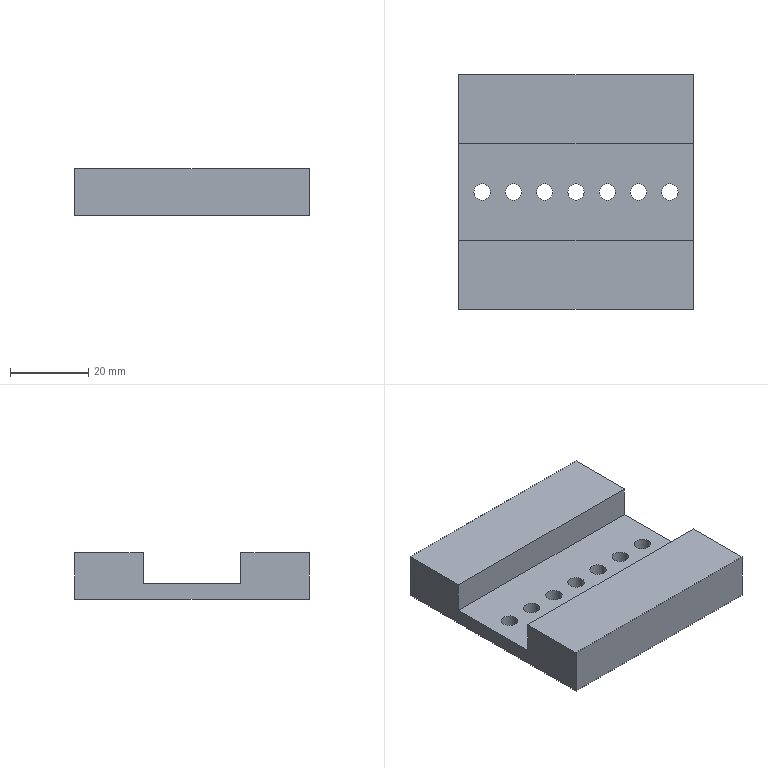Part | SolidWorks | features 3DProfileFeature 1, Extrusion 1, HoleWzd 1, ICE 1, LPattern 1, MirrorPattern 1 | 1 solid | 24 faces | box 60 x 60 x 12 mm | volume 30812 mm3 | cylinder 14 | plane 10 | commonest cylinder face diameters 4.2 x14
STEP:
#1=CARTESIAN_POINT('',(21.9,0.,0.));
#2=VERTEX_POINT('',#1);
#3=CARTESIAN_POINT('',(26.1,0.,0.));
#4=VERTEX_POINT('',#3);
#5=CARTESIAN_POINT('',(24.,0.,0.));
#6=DIRECTION('',(0.,0.,1.));
#7=DIRECTION('',(1.,0.,0.));
#8=AXIS2_PLACEMENT_3D('',#5,#6,#7);
#9=CIRCLE('',#8,2.1);
#10=EDGE_CURVE('',#2,#4,#9,.T.);
#11=ORIENTED_EDGE('',*,*,#10,.F.);
#12=CARTESIAN_POINT('',(21.9,0.,4.));
#13=VERTEX_POINT('',#12);
#14=CARTESIAN_POINT('',(21.9,0.,4.));
#15=DIRECTION('',(0.,0.,1.));
#16=VECTOR('',#15,1000.);
#17=LINE('',#14,#16);
#18=EDGE_CURVE('',#2,#13,#17,.T.);
#19=ORIENTED_EDGE('',*,*,#18,.T.);
#20=CARTESIAN_POINT('',(26.1,0.,4.));
#21=VERTEX_POINT('',#20);
#22=CARTESIAN_POINT('',(24.,0.,4.));
#23=DIRECTION('',(0.,0.,1.));
#24=DIRECTION('',(1.,0.,0.));
#25=AXIS2_PLACEMENT_3D('',#22,#23,#24);
#26=CIRCLE('',#25,2.1);
#27=EDGE_CURVE('',#13,#21,#26,.T.);
#28=ORIENTED_EDGE('',*,*,#27,.T.);
#29=CARTESIAN_POINT('',(26.1,0.,4.));
#30=DIRECTION('',(0.,0.,1.));
#31=VECTOR('',#30,1000.);
#32=LINE('',#29,#31);
#33=EDGE_CURVE('',#4,#21,#32,.T.);
#34=ORIENTED_EDGE('',*,*,#33,.F.);
#35=EDGE_LOOP('',(#11,#19,#28,#34));
#36=FACE_OUTER_BOUND('',#35,.T.);
#37=CARTESIAN_POINT('',(24.,0.,4.));
#38=DIRECTION('',(0.,0.,1.));
#39=DIRECTION('',(1.,0.,0.));
#40=AXIS2_PLACEMENT_3D('',#37,#38,#39);
#41=CYLINDRICAL_SURFACE('',#40,2.1);
#42=ADVANCED_FACE('',(#36),#41,.F.);
#43=CARTESIAN_POINT('',(13.9,0.,0.));
#44=VERTEX_POINT('',#43);
#45=CARTESIAN_POINT('',(18.1,0.,0.));
#46=VERTEX_POINT('',#45);
#47=CARTESIAN_POINT('',(16.,0.,0.));
#48=DIRECTION('',(0.,0.,1.));
#49=DIRECTION('',(1.,0.,0.));
#50=AXIS2_PLACEMENT_3D('',#47,#48,#49);
#51=CIRCLE('',#50,2.1);
#52=EDGE_CURVE('',#44,#46,#51,.T.);
#53=ORIENTED_EDGE('',*,*,#52,.F.);
#54=CARTESIAN_POINT('',(13.9,0.,4.));
#55=VERTEX_POINT('',#54);
#56=CARTESIAN_POINT('',(13.9,0.,4.));
#57=DIRECTION('',(0.,0.,1.));
#58=VECTOR('',#57,1000.);
#59=LINE('',#56,#58);
#60=EDGE_CURVE('',#44,#55,#59,.T.);
#61=ORIENTED_EDGE('',*,*,#60,.T.);
#62=CARTESIAN_POINT('',(18.1,0.,4.));
#63=VERTEX_POINT('',#62);
#64=CARTESIAN_POINT('',(16.,0.,4.));
#65=DIRECTION('',(0.,0.,1.));
#66=DIRECTION('',(1.,0.,0.));
#67=AXIS2_PLACEMENT_3D('',#64,#65,#66);
#68=CIRCLE('',#67,2.1);
#69=EDGE_CURVE('',#55,#63,#68,.T.);
#70=ORIENTED_EDGE('',*,*,#69,.T.);
#71=CARTESIAN_POINT('',(18.1,0.,4.));
#72=DIRECTION('',(0.,0.,1.));
#73=VECTOR('',#72,1000.);
#74=LINE('',#71,#73);
#75=EDGE_CURVE('',#46,#63,#74,.T.);
#76=ORIENTED_EDGE('',*,*,#75,.F.);
#77=EDGE_LOOP('',(#53,#61,#70,#76));
#78=FACE_OUTER_BOUND('',#77,.T.);
#79=CARTESIAN_POINT('',(16.,0.,4.));
#80=DIRECTION('',(0.,0.,1.));
#81=DIRECTION('',(1.,0.,0.));
#82=AXIS2_PLACEMENT_3D('',#79,#80,#81);
#83=CYLINDRICAL_SURFACE('',#82,2.1);
#84=ADVANCED_FACE('',(#78),#83,.F.);
#85=CARTESIAN_POINT('',(5.9,0.,0.));
#86=VERTEX_POINT('',#85);
#87=CARTESIAN_POINT('',(10.1,0.,0.));
#88=VERTEX_POINT('',#87);
#89=CARTESIAN_POINT('',(8.,0.,0.));
#90=DIRECTION('',(0.,0.,1.));
#91=DIRECTION('',(1.,0.,0.));
#92=AXIS2_PLACEMENT_3D('',#89,#90,#91);
#93=CIRCLE('',#92,2.1);
#94=EDGE_CURVE('',#86,#88,#93,.T.);
#95=ORIENTED_EDGE('',*,*,#94,.F.);
#96=CARTESIAN_POINT('',(5.9,0.,4.));
#97=VERTEX_POINT('',#96);
#98=CARTESIAN_POINT('',(5.9,0.,4.));
#99=DIRECTION('',(0.,0.,1.));
#100=VECTOR('',#99,1000.);
#101=LINE('',#98,#100);
#102=EDGE_CURVE('',#86,#97,#101,.T.);
#103=ORIENTED_EDGE('',*,*,#102,.T.);
#104=CARTESIAN_POINT('',(10.1,0.,4.));
#105=VERTEX_POINT('',#104);
#106=CARTESIAN_POINT('',(8.,0.,4.));
#107=DIRECTION('',(0.,0.,1.));
#108=DIRECTION('',(1.,0.,0.));
#109=AXIS2_PLACEMENT_3D('',#106,#107,#108);
#110=CIRCLE('',#109,2.1);
#111=EDGE_CURVE('',#97,#105,#110,.T.);
#112=ORIENTED_EDGE('',*,*,#111,.T.);
#113=CARTESIAN_POINT('',(10.1,0.,4.));
#114=DIRECTION('',(0.,0.,1.));
#115=VECTOR('',#114,1000.);
#116=LINE('',#113,#115);
#117=EDGE_CURVE('',#88,#105,#116,.T.);
#118=ORIENTED_EDGE('',*,*,#117,.F.);
#119=EDGE_LOOP('',(#95,#103,#112,#118));
#120=FACE_OUTER_BOUND('',#119,.T.);
#121=CARTESIAN_POINT('',(8.,0.,4.));
#122=DIRECTION('',(0.,0.,1.));
#123=DIRECTION('',(1.,0.,0.));
#124=AXIS2_PLACEMENT_3D('',#121,#122,#123);
#125=CYLINDRICAL_SURFACE('',#124,2.1);
#126=ADVANCED_FACE('',(#120),#125,.F.);
#127=CARTESIAN_POINT('',(-26.1,0.,0.));
#128=VERTEX_POINT('',#127);
#129=CARTESIAN_POINT('',(-21.9,0.,0.));
#130=VERTEX_POINT('',#129);
#131=CARTESIAN_POINT('',(-24.,0.,0.));
#132=DIRECTION('',(0.,0.,1.));
#133=DIRECTION('',(1.,0.,0.));
#134=AXIS2_PLACEMENT_3D('',#131,#132,#133);
#135=CIRCLE('',#134,2.1);
#136=EDGE_CURVE('',#128,#130,#135,.T.);
#137=ORIENTED_EDGE('',*,*,#136,.F.);
#138=CARTESIAN_POINT('',(-26.1,0.,4.));
#139=VERTEX_POINT('',#138);
#140=CARTESIAN_POINT('',(-26.1,0.,4.));
#141=DIRECTION('',(0.,0.,1.));
#142=VECTOR('',#141,1000.);
#143=LINE('',#140,#142);
#144=EDGE_CURVE('',#128,#139,#143,.T.);
#145=ORIENTED_EDGE('',*,*,#144,.T.);
#146=CARTESIAN_POINT('',(-21.9,0.,4.));
#147=VERTEX_POINT('',#146);
#148=CARTESIAN_POINT('',(-24.,0.,4.));
#149=DIRECTION('',(0.,0.,1.));
#150=DIRECTION('',(1.,0.,0.));
#151=AXIS2_PLACEMENT_3D('',#148,#149,#150);
#152=CIRCLE('',#151,2.1);
#153=EDGE_CURVE('',#139,#147,#152,.T.);
#154=ORIENTED_EDGE('',*,*,#153,.T.);
#155=CARTESIAN_POINT('',(-21.9,0.,4.));
#156=DIRECTION('',(0.,0.,1.));
#157=VECTOR('',#156,1000.);
#158=LINE('',#155,#157);
#159=EDGE_CURVE('',#130,#147,#158,.T.);
#160=ORIENTED_EDGE('',*,*,#159,.F.);
#161=EDGE_LOOP('',(#137,#145,#154,#160));
#162=FACE_OUTER_BOUND('',#161,.T.);
#163=CARTESIAN_POINT('',(-24.,0.,4.));
#164=DIRECTION('',(0.,0.,1.));
#165=DIRECTION('',(1.,0.,0.));
#166=AXIS2_PLACEMENT_3D('',#163,#164,#165);
#167=CYLINDRICAL_SURFACE('',#166,2.1);
#168=ADVANCED_FACE('',(#162),#167,.F.);
#169=CARTESIAN_POINT('',(-18.1,0.,0.));
#170=VERTEX_POINT('',#169);
#171=CARTESIAN_POINT('',(-13.9,0.,0.));
#172=VERTEX_POINT('',#171);
#173=CARTESIAN_POINT('',(-16.,0.,0.));
#174=DIRECTION('',(0.,0.,1.));
#175=DIRECTION('',(1.,0.,0.));
#176=AXIS2_PLACEMENT_3D('',#173,#174,#175);
#177=CIRCLE('',#176,2.1);
#178=EDGE_CURVE('',#170,#172,#177,.T.);
#179=ORIENTED_EDGE('',*,*,#178,.F.);
#180=CARTESIAN_POINT('',(-18.1,0.,4.));
#181=VERTEX_POINT('',#180);
#182=CARTESIAN_POINT('',(-18.1,0.,4.));
#183=DIRECTION('',(0.,0.,1.));
#184=VECTOR('',#183,1000.);
#185=LINE('',#182,#184);
#186=EDGE_CURVE('',#170,#181,#185,.T.);
#187=ORIENTED_EDGE('',*,*,#186,.T.);
#188=CARTESIAN_POINT('',(-13.9,0.,4.));
#189=VERTEX_POINT('',#188);
#190=CARTESIAN_POINT('',(-16.,0.,4.));
#191=DIRECTION('',(0.,0.,1.));
#192=DIRECTION('',(1.,0.,0.));
#193=AXIS2_PLACEMENT_3D('',#190,#191,#192);
#194=CIRCLE('',#193,2.1);
#195=EDGE_CURVE('',#181,#189,#194,.T.);
#196=ORIENTED_EDGE('',*,*,#195,.T.);
#197=CARTESIAN_POINT('',(-13.9,0.,4.));
#198=DIRECTION('',(0.,0.,1.));
#199=VECTOR('',#198,1000.);
#200=LINE('',#197,#199);
#201=EDGE_CURVE('',#172,#189,#200,.T.);
#202=ORIENTED_EDGE('',*,*,#201,.F.);
#203=EDGE_LOOP('',(#179,#187,#196,#202));
#204=FACE_OUTER_BOUND('',#203,.T.);
#205=CARTESIAN_POINT('',(-16.,0.,4.));
#206=DIRECTION('',(0.,0.,1.));
#207=DIRECTION('',(1.,0.,0.));
#208=AXIS2_PLACEMENT_3D('',#205,#206,#207);
#209=CYLINDRICAL_SURFACE('',#208,2.1);
#210=ADVANCED_FACE('',(#204),#209,.F.);
#211=CARTESIAN_POINT('',(-10.1,0.,0.));
#212=VERTEX_POINT('',#211);
#213=CARTESIAN_POINT('',(-5.9,0.,0.));
#214=VERTEX_POINT('',#213);
#215=CARTESIAN_POINT('',(-8.,0.,0.));
#216=DIRECTION('',(0.,0.,1.));
#217=DIRECTION('',(1.,0.,0.));
#218=AXIS2_PLACEMENT_3D('',#215,#216,#217);
#219=CIRCLE('',#218,2.1);
#220=EDGE_CURVE('',#212,#214,#219,.T.);
#221=ORIENTED_EDGE('',*,*,#220,.F.);
#222=CARTESIAN_POINT('',(-10.1,0.,4.));
#223=VERTEX_POINT('',#222);
#224=CARTESIAN_POINT('',(-10.1,0.,4.));
#225=DIRECTION('',(0.,0.,1.));
#226=VECTOR('',#225,1000.);
#227=LINE('',#224,#226);
#228=EDGE_CURVE('',#212,#223,#227,.T.);
#229=ORIENTED_EDGE('',*,*,#228,.T.);
#230=CARTESIAN_POINT('',(-5.9,0.,4.));
#231=VERTEX_POINT('',#230);
#232=CARTESIAN_POINT('',(-8.,0.,4.));
#233=DIRECTION('',(0.,0.,1.));
#234=DIRECTION('',(1.,0.,0.));
#235=AXIS2_PLACEMENT_3D('',#232,#233,#234);
#236=CIRCLE('',#235,2.1);
#237=EDGE_CURVE('',#223,#231,#236,.T.);
#238=ORIENTED_EDGE('',*,*,#237,.T.);
#239=CARTESIAN_POINT('',(-5.9,0.,4.));
#240=DIRECTION('',(0.,0.,1.));
#241=VECTOR('',#240,1000.);
#242=LINE('',#239,#241);
#243=EDGE_CURVE('',#214,#231,#242,.T.);
#244=ORIENTED_EDGE('',*,*,#243,.F.);
#245=EDGE_LOOP('',(#221,#229,#238,#244));
#246=FACE_OUTER_BOUND('',#245,.T.);
#247=CARTESIAN_POINT('',(-8.,0.,4.));
#248=DIRECTION('',(0.,0.,1.));
#249=DIRECTION('',(1.,0.,0.));
#250=AXIS2_PLACEMENT_3D('',#247,#248,#249);
#251=CYLINDRICAL_SURFACE('',#250,2.1);
#252=ADVANCED_FACE('',(#246),#251,.F.);
#253=CARTESIAN_POINT('',(-2.1,0.,0.));
#254=VERTEX_POINT('',#253);
#255=CARTESIAN_POINT('',(2.1,0.,0.));
#256=VERTEX_POINT('',#255);
#257=CARTESIAN_POINT('',(0.,0.,0.));
#258=DIRECTION('',(0.,0.,1.));
#259=DIRECTION('',(1.,0.,0.));
#260=AXIS2_PLACEMENT_3D('',#257,#258,#259);
#261=CIRCLE('',#260,2.1);
#262=EDGE_CURVE('',#254,#256,#261,.T.);
#263=ORIENTED_EDGE('',*,*,#262,.F.);
#264=CARTESIAN_POINT('',(-2.1,0.,4.));
#265=VERTEX_POINT('',#264);
#266=CARTESIAN_POINT('',(-2.1,0.,4.));
#267=DIRECTION('',(0.,0.,1.));
#268=VECTOR('',#267,1000.);
#269=LINE('',#266,#268);
#270=EDGE_CURVE('',#254,#265,#269,.T.);
#271=ORIENTED_EDGE('',*,*,#270,.T.);
#272=CARTESIAN_POINT('',(2.1,0.,4.));
#273=VERTEX_POINT('',#272);
#274=CARTESIAN_POINT('',(0.,0.,4.));
#275=DIRECTION('',(0.,0.,1.));
#276=DIRECTION('',(1.,0.,0.));
#277=AXIS2_PLACEMENT_3D('',#274,#275,#276);
#278=CIRCLE('',#277,2.1);
#279=EDGE_CURVE('',#265,#273,#278,.T.);
#280=ORIENTED_EDGE('',*,*,#279,.T.);
#281=CARTESIAN_POINT('',(2.1,0.,4.));
#282=DIRECTION('',(0.,0.,1.));
#283=VECTOR('',#282,1000.);
#284=LINE('',#281,#283);
#285=EDGE_CURVE('',#256,#273,#284,.T.);
#286=ORIENTED_EDGE('',*,*,#285,.F.);
#287=EDGE_LOOP('',(#263,#271,#280,#286));
#288=FACE_OUTER_BOUND('',#287,.T.);
#289=CARTESIAN_POINT('',(0.,0.,4.));
#290=DIRECTION('',(0.,0.,1.));
#291=DIRECTION('',(1.,0.,0.));
#292=AXIS2_PLACEMENT_3D('',#289,#290,#291);
#293=CYLINDRICAL_SURFACE('',#292,2.1);
#294=ADVANCED_FACE('',(#288),#293,.F.);
#295=CARTESIAN_POINT('',(16.,0.,4.));
#296=DIRECTION('',(0.,0.,1.));
#297=DIRECTION('',(1.,0.,0.));
#298=AXIS2_PLACEMENT_3D('',#295,#296,#297);
#299=CIRCLE('',#298,2.1);
#300=EDGE_CURVE('',#63,#55,#299,.T.);
#301=ORIENTED_EDGE('',*,*,#300,.F.);
#302=ORIENTED_EDGE('',*,*,#69,.F.);
#303=EDGE_LOOP('',(#301,#302));
#304=FACE_BOUND('',#303,.T.);
#305=CARTESIAN_POINT('',(8.,0.,4.));
#306=DIRECTION('',(0.,0.,1.));
#307=DIRECTION('',(1.,0.,0.));
#308=AXIS2_PLACEMENT_3D('',#305,#306,#307);
#309=CIRCLE('',#308,2.1);
#310=EDGE_CURVE('',#105,#97,#309,.T.);
#311=ORIENTED_EDGE('',*,*,#310,.F.);
#312=ORIENTED_EDGE('',*,*,#111,.F.);
#313=EDGE_LOOP('',(#311,#312));
#314=FACE_BOUND('',#313,.T.);
#315=CARTESIAN_POINT('',(-24.,0.,4.));
#316=DIRECTION('',(0.,0.,1.));
#317=DIRECTION('',(1.,0.,0.));
#318=AXIS2_PLACEMENT_3D('',#315,#316,#317);
#319=CIRCLE('',#318,2.1);
#320=EDGE_CURVE('',#147,#139,#319,.T.);
#321=ORIENTED_EDGE('',*,*,#320,.F.);
#322=ORIENTED_EDGE('',*,*,#153,.F.);
#323=EDGE_LOOP('',(#321,#322));
#324=FACE_BOUND('',#323,.T.);
#325=CARTESIAN_POINT('',(-16.,0.,4.));
#326=DIRECTION('',(0.,0.,1.));
#327=DIRECTION('',(1.,0.,0.));
#328=AXIS2_PLACEMENT_3D('',#325,#326,#327);
#329=CIRCLE('',#328,2.1);
#330=EDGE_CURVE('',#189,#181,#329,.T.);
#331=ORIENTED_EDGE('',*,*,#330,.F.);
#332=ORIENTED_EDGE('',*,*,#195,.F.);
#333=EDGE_LOOP('',(#331,#332));
#334=FACE_BOUND('',#333,.T.);
#335=CARTESIAN_POINT('',(-8.,0.,4.));
#336=DIRECTION('',(0.,0.,1.));
#337=DIRECTION('',(1.,0.,0.));
#338=AXIS2_PLACEMENT_3D('',#335,#336,#337);
#339=CIRCLE('',#338,2.1);
#340=EDGE_CURVE('',#231,#223,#339,.T.);
#341=ORIENTED_EDGE('',*,*,#340,.F.);
#342=ORIENTED_EDGE('',*,*,#237,.F.);
#343=EDGE_LOOP('',(#341,#342));
#344=FACE_BOUND('',#343,.T.);
#345=CARTESIAN_POINT('',(0.,0.,4.));
#346=DIRECTION('',(0.,0.,1.));
#347=DIRECTION('',(1.,0.,0.));
#348=AXIS2_PLACEMENT_3D('',#345,#346,#347);
#349=CIRCLE('',#348,2.1);
#350=EDGE_CURVE('',#273,#265,#349,.T.);
#351=ORIENTED_EDGE('',*,*,#350,.F.);
#352=ORIENTED_EDGE('',*,*,#279,.F.);
#353=EDGE_LOOP('',(#351,#352));
#354=FACE_BOUND('',#353,.T.);
#355=CARTESIAN_POINT('',(30.,-12.5,4.));
#356=VERTEX_POINT('',#355);
#357=CARTESIAN_POINT('',(30.,12.5,4.));
#358=VERTEX_POINT('',#357);
#359=CARTESIAN_POINT('',(30.,-12.5,4.));
#360=DIRECTION('',(0.,1.,0.));
#361=VECTOR('',#360,1000.);
#362=LINE('',#359,#361);
#363=EDGE_CURVE('',#356,#358,#362,.T.);
#364=ORIENTED_EDGE('',*,*,#363,.T.);
#365=CARTESIAN_POINT('',(-30.,12.5,4.));
#366=VERTEX_POINT('',#365);
#367=CARTESIAN_POINT('',(-30.,12.5,4.));
#368=DIRECTION('',(-1.,0.,0.));
#369=VECTOR('',#368,1000.);
#370=LINE('',#367,#369);
#371=EDGE_CURVE('',#358,#366,#370,.T.);
#372=ORIENTED_EDGE('',*,*,#371,.T.);
#373=CARTESIAN_POINT('',(-30.,-12.5,4.));
#374=VERTEX_POINT('',#373);
#375=CARTESIAN_POINT('',(-30.,-12.5,4.));
#376=DIRECTION('',(0.,-1.,0.));
#377=VECTOR('',#376,1000.);
#378=LINE('',#375,#377);
#379=EDGE_CURVE('',#366,#374,#378,.T.);
#380=ORIENTED_EDGE('',*,*,#379,.T.);
#381=CARTESIAN_POINT('',(-30.,-12.5,4.));
#382=DIRECTION('',(1.,0.,0.));
#383=VECTOR('',#382,1000.);
#384=LINE('',#381,#383);
#385=EDGE_CURVE('',#374,#356,#384,.T.);
#386=ORIENTED_EDGE('',*,*,#385,.T.);
#387=EDGE_LOOP('',(#364,#372,#380,#386));
#388=FACE_OUTER_BOUND('',#387,.T.);
#389=CARTESIAN_POINT('',(24.,0.,4.));
#390=DIRECTION('',(0.,0.,1.));
#391=DIRECTION('',(1.,0.,0.));
#392=AXIS2_PLACEMENT_3D('',#389,#390,#391);
#393=CIRCLE('',#392,2.1);
#394=EDGE_CURVE('',#21,#13,#393,.T.);
#395=ORIENTED_EDGE('',*,*,#394,.F.);
#396=ORIENTED_EDGE('',*,*,#27,.F.);
#397=EDGE_LOOP('',(#395,#396));
#398=FACE_BOUND('',#397,.T.);
#399=CARTESIAN_POINT('',(0.,0.,4.));
#400=DIRECTION('',(0.,0.,-1.));
#401=DIRECTION('',(-1.,0.,0.));
#402=AXIS2_PLACEMENT_3D('',#399,#400,#401);
#403=PLANE('',#402);
#404=ADVANCED_FACE('',(#304,#314,#324,#334,#344,#354,#388,#398),#403,.F.);
#405=CARTESIAN_POINT('',(30.,-30.,12.));
#406=VERTEX_POINT('',#405);
#407=CARTESIAN_POINT('',(30.,-12.5,12.));
#408=VERTEX_POINT('',#407);
#409=CARTESIAN_POINT('',(30.,-30.,12.));
#410=DIRECTION('',(0.,1.,0.));
#411=VECTOR('',#410,1000.);
#412=LINE('',#409,#411);
#413=EDGE_CURVE('',#406,#408,#412,.T.);
#414=ORIENTED_EDGE('',*,*,#413,.T.);
#415=CARTESIAN_POINT('',(-30.,-12.5,12.));
#416=VERTEX_POINT('',#415);
#417=CARTESIAN_POINT('',(-30.,-12.5,12.));
#418=DIRECTION('',(1.,0.,0.));
#419=VECTOR('',#418,1000.);
#420=LINE('',#417,#419);
#421=EDGE_CURVE('',#416,#408,#420,.T.);
#422=ORIENTED_EDGE('',*,*,#421,.F.);
#423=CARTESIAN_POINT('',(-30.,-30.,12.));
#424=VERTEX_POINT('',#423);
#425=CARTESIAN_POINT('',(-30.,-30.,12.));
#426=DIRECTION('',(0.,-1.,0.));
#427=VECTOR('',#426,1000.);
#428=LINE('',#425,#427);
#429=EDGE_CURVE('',#416,#424,#428,.T.);
#430=ORIENTED_EDGE('',*,*,#429,.T.);
#431=CARTESIAN_POINT('',(-30.,-30.,12.));
#432=DIRECTION('',(1.,0.,0.));
#433=VECTOR('',#432,1000.);
#434=LINE('',#431,#433);
#435=EDGE_CURVE('',#424,#406,#434,.T.);
#436=ORIENTED_EDGE('',*,*,#435,.T.);
#437=EDGE_LOOP('',(#414,#422,#430,#436));
#438=FACE_OUTER_BOUND('',#437,.T.);
#439=CARTESIAN_POINT('',(0.,0.,12.));
#440=DIRECTION('',(0.,0.,-1.));
#441=DIRECTION('',(-1.,0.,0.));
#442=AXIS2_PLACEMENT_3D('',#439,#440,#441);
#443=PLANE('',#442);
#444=ADVANCED_FACE('',(#438),#443,.F.);
#445=ORIENTED_EDGE('',*,*,#363,.F.);
#446=CARTESIAN_POINT('',(30.,-12.5,4.));
#447=DIRECTION('',(0.,0.,1.));
#448=VECTOR('',#447,1000.);
#449=LINE('',#446,#448);
#450=EDGE_CURVE('',#356,#408,#449,.T.);
#451=ORIENTED_EDGE('',*,*,#450,.T.);
#452=ORIENTED_EDGE('',*,*,#413,.F.);
#453=CARTESIAN_POINT('',(30.,-30.,0.));
#454=VERTEX_POINT('',#453);
#455=CARTESIAN_POINT('',(30.,-30.,12.));
#456=DIRECTION('',(0.,0.,-1.));
#457=VECTOR('',#456,1000.);
#458=LINE('',#455,#457);
#459=EDGE_CURVE('',#406,#454,#458,.T.);
#460=ORIENTED_EDGE('',*,*,#459,.T.);
#461=CARTESIAN_POINT('',(30.,30.,0.));
#462=VERTEX_POINT('',#461);
#463=CARTESIAN_POINT('',(30.,-30.,0.));
#464=DIRECTION('',(0.,1.,0.));
#465=VECTOR('',#464,1000.);
#466=LINE('',#463,#465);
#467=EDGE_CURVE('',#454,#462,#466,.T.);
#468=ORIENTED_EDGE('',*,*,#467,.T.);
#469=CARTESIAN_POINT('',(30.,30.,12.));
#470=VERTEX_POINT('',#469);
#471=CARTESIAN_POINT('',(30.,30.,12.));
#472=DIRECTION('',(0.,0.,-1.));
#473=VECTOR('',#472,1000.);
#474=LINE('',#471,#473);
#475=EDGE_CURVE('',#470,#462,#474,.T.);
#476=ORIENTED_EDGE('',*,*,#475,.F.);
#477=CARTESIAN_POINT('',(30.,12.5,12.));
#478=VERTEX_POINT('',#477);
#479=CARTESIAN_POINT('',(30.,-30.,12.));
#480=DIRECTION('',(0.,1.,0.));
#481=VECTOR('',#480,1000.);
#482=LINE('',#479,#481);
#483=EDGE_CURVE('',#478,#470,#482,.T.);
#484=ORIENTED_EDGE('',*,*,#483,.F.);
#485=CARTESIAN_POINT('',(30.,12.5,4.));
#486=DIRECTION('',(0.,0.,1.));
#487=VECTOR('',#486,1000.);
#488=LINE('',#485,#487);
#489=EDGE_CURVE('',#358,#478,#488,.T.);
#490=ORIENTED_EDGE('',*,*,#489,.F.);
#491=EDGE_LOOP('',(#445,#451,#452,#460,#468,#476,#484,#490));
#492=FACE_OUTER_BOUND('',#491,.T.);
#493=CARTESIAN_POINT('',(30.,-30.,12.));
#494=DIRECTION('',(-1.,0.,0.));
#495=DIRECTION('',(0.,0.,1.));
#496=AXIS2_PLACEMENT_3D('',#493,#494,#495);
#497=PLANE('',#496);
#498=ADVANCED_FACE('',(#492),#497,.F.);
#499=CARTESIAN_POINT('',(-30.,30.,0.));
#500=VERTEX_POINT('',#499);
#501=CARTESIAN_POINT('',(-30.,30.,0.));
#502=DIRECTION('',(-1.,0.,0.));
#503=VECTOR('',#502,1000.);
#504=LINE('',#501,#503);
#505=EDGE_CURVE('',#462,#500,#504,.T.);
#506=ORIENTED_EDGE('',*,*,#505,.T.);
#507=CARTESIAN_POINT('',(-30.,30.,12.));
#508=VERTEX_POINT('',#507);
#509=CARTESIAN_POINT('',(-30.,30.,12.));
#510=DIRECTION('',(0.,0.,-1.));
#511=VECTOR('',#510,1000.);
#512=LINE('',#509,#511);
#513=EDGE_CURVE('',#508,#500,#512,.T.);
#514=ORIENTED_EDGE('',*,*,#513,.F.);
#515=CARTESIAN_POINT('',(-30.,30.,12.));
#516=DIRECTION('',(-1.,0.,0.));
#517=VECTOR('',#516,1000.);
#518=LINE('',#515,#517);
#519=EDGE_CURVE('',#470,#508,#518,.T.);
#520=ORIENTED_EDGE('',*,*,#519,.F.);
#521=ORIENTED_EDGE('',*,*,#475,.T.);
#522=EDGE_LOOP('',(#506,#514,#520,#521));
#523=FACE_OUTER_BOUND('',#522,.T.);
#524=CARTESIAN_POINT('',(-30.,30.,12.));
#525=DIRECTION('',(0.,-1.,0.));
#526=DIRECTION('',(0.,0.,-1.));
#527=AXIS2_PLACEMENT_3D('',#524,#525,#526);
#528=PLANE('',#527);
#529=ADVANCED_FACE('',(#523),#528,.F.);
#530=ORIENTED_EDGE('',*,*,#429,.F.);
#531=CARTESIAN_POINT('',(-30.,-12.5,4.));
#532=DIRECTION('',(0.,0.,1.));
#533=VECTOR('',#532,1000.);
#534=LINE('',#531,#533);
#535=EDGE_CURVE('',#374,#416,#534,.T.);
#536=ORIENTED_EDGE('',*,*,#535,.F.);
#537=ORIENTED_EDGE('',*,*,#379,.F.);
#538=CARTESIAN_POINT('',(-30.,12.5,12.));
#539=VERTEX_POINT('',#538);
#540=CARTESIAN_POINT('',(-30.,12.5,4.));
#541=DIRECTION('',(0.,0.,1.));
#542=VECTOR('',#541,1000.);
#543=LINE('',#540,#542);
#544=EDGE_CURVE('',#366,#539,#543,.T.);
#545=ORIENTED_EDGE('',*,*,#544,.T.);
#546=CARTESIAN_POINT('',(-30.,-30.,12.));
#547=DIRECTION('',(0.,-1.,0.));
#548=VECTOR('',#547,1000.);
#549=LINE('',#546,#548);
#550=EDGE_CURVE('',#508,#539,#549,.T.);
#551=ORIENTED_EDGE('',*,*,#550,.F.);
#552=ORIENTED_EDGE('',*,*,#513,.T.);
#553=CARTESIAN_POINT('',(-30.,-30.,0.));
#554=VERTEX_POINT('',#553);
#555=CARTESIAN_POINT('',(-30.,-30.,0.));
#556=DIRECTION('',(0.,-1.,0.));
#557=VECTOR('',#556,1000.);
#558=LINE('',#555,#557);
#559=EDGE_CURVE('',#500,#554,#558,.T.);
#560=ORIENTED_EDGE('',*,*,#559,.T.);
#561=CARTESIAN_POINT('',(-30.,-30.,12.));
#562=DIRECTION('',(0.,0.,-1.));
#563=VECTOR('',#562,1000.);
#564=LINE('',#561,#563);
#565=EDGE_CURVE('',#424,#554,#564,.T.);
#566=ORIENTED_EDGE('',*,*,#565,.F.);
#567=EDGE_LOOP('',(#530,#536,#537,#545,#551,#552,#560,#566));
#568=FACE_OUTER_BOUND('',#567,.T.);
#569=CARTESIAN_POINT('',(-30.,-30.,12.));
#570=DIRECTION('',(1.,0.,0.));
#571=DIRECTION('',(0.,0.,-1.));
#572=AXIS2_PLACEMENT_3D('',#569,#570,#571);
#573=PLANE('',#572);
#574=ADVANCED_FACE('',(#568),#573,.F.);
#575=CARTESIAN_POINT('',(-30.,-30.,0.));
#576=DIRECTION('',(1.,0.,0.));
#577=VECTOR('',#576,1000.);
#578=LINE('',#575,#577);
#579=EDGE_CURVE('',#554,#454,#578,.T.);
#580=ORIENTED_EDGE('',*,*,#579,.T.);
#581=ORIENTED_EDGE('',*,*,#459,.F.);
#582=ORIENTED_EDGE('',*,*,#435,.F.);
#583=ORIENTED_EDGE('',*,*,#565,.T.);
#584=EDGE_LOOP('',(#580,#581,#582,#583));
#585=FACE_OUTER_BOUND('',#584,.T.);
#586=CARTESIAN_POINT('',(-30.,-30.,12.));
#587=DIRECTION('',(0.,1.,0.));
#588=DIRECTION('',(0.,0.,1.));
#589=AXIS2_PLACEMENT_3D('',#586,#587,#588);
#590=PLANE('',#589);
#591=ADVANCED_FACE('',(#585),#590,.F.);
#592=ORIENTED_EDGE('',*,*,#550,.T.);
#593=CARTESIAN_POINT('',(-30.,12.5,12.));
#594=DIRECTION('',(-1.,0.,0.));
#595=VECTOR('',#594,1000.);
#596=LINE('',#593,#595);
#597=EDGE_CURVE('',#478,#539,#596,.T.);
#598=ORIENTED_EDGE('',*,*,#597,.F.);
#599=ORIENTED_EDGE('',*,*,#483,.T.);
#600=ORIENTED_EDGE('',*,*,#519,.T.);
#601=EDGE_LOOP('',(#592,#598,#599,#600));
#602=FACE_OUTER_BOUND('',#601,.T.);
#603=CARTESIAN_POINT('',(0.,0.,12.));
#604=DIRECTION('',(0.,0.,-1.));
#605=DIRECTION('',(-1.,0.,0.));
#606=AXIS2_PLACEMENT_3D('',#603,#604,#605);
#607=PLANE('',#606);
#608=ADVANCED_FACE('',(#602),#607,.F.);
#609=CARTESIAN_POINT('',(24.,0.,0.));
#610=DIRECTION('',(0.,0.,1.));
#611=DIRECTION('',(1.,0.,0.));
#612=AXIS2_PLACEMENT_3D('',#609,#610,#611);
#613=CIRCLE('',#612,2.1);
#614=EDGE_CURVE('',#4,#2,#613,.T.);
#615=ORIENTED_EDGE('',*,*,#614,.T.);
#616=ORIENTED_EDGE('',*,*,#10,.T.);
#617=EDGE_LOOP('',(#615,#616));
#618=FACE_BOUND('',#617,.T.);
#619=CARTESIAN_POINT('',(16.,0.,0.));
#620=DIRECTION('',(0.,0.,1.));
#621=DIRECTION('',(1.,0.,0.));
#622=AXIS2_PLACEMENT_3D('',#619,#620,#621);
#623=CIRCLE('',#622,2.1);
#624=EDGE_CURVE('',#46,#44,#623,.T.);
#625=ORIENTED_EDGE('',*,*,#624,.T.);
#626=ORIENTED_EDGE('',*,*,#52,.T.);
#627=EDGE_LOOP('',(#625,#626));
#628=FACE_BOUND('',#627,.T.);
#629=CARTESIAN_POINT('',(8.,0.,0.));
#630=DIRECTION('',(0.,0.,1.));
#631=DIRECTION('',(1.,0.,0.));
#632=AXIS2_PLACEMENT_3D('',#629,#630,#631);
#633=CIRCLE('',#632,2.1);
#634=EDGE_CURVE('',#88,#86,#633,.T.);
#635=ORIENTED_EDGE('',*,*,#634,.T.);
#636=ORIENTED_EDGE('',*,*,#94,.T.);
#637=EDGE_LOOP('',(#635,#636));
#638=FACE_BOUND('',#637,.T.);
#639=CARTESIAN_POINT('',(-24.,0.,0.));
#640=DIRECTION('',(0.,0.,1.));
#641=DIRECTION('',(1.,0.,0.));
#642=AXIS2_PLACEMENT_3D('',#639,#640,#641);
#643=CIRCLE('',#642,2.1);
#644=EDGE_CURVE('',#130,#128,#643,.T.);
#645=ORIENTED_EDGE('',*,*,#644,.T.);
#646=ORIENTED_EDGE('',*,*,#136,.T.);
#647=EDGE_LOOP('',(#645,#646));
#648=FACE_BOUND('',#647,.T.);
#649=CARTESIAN_POINT('',(-16.,0.,0.));
#650=DIRECTION('',(0.,0.,1.));
#651=DIRECTION('',(1.,0.,0.));
#652=AXIS2_PLACEMENT_3D('',#649,#650,#651);
#653=CIRCLE('',#652,2.1);
#654=EDGE_CURVE('',#172,#170,#653,.T.);
#655=ORIENTED_EDGE('',*,*,#654,.T.);
#656=ORIENTED_EDGE('',*,*,#178,.T.);
#657=EDGE_LOOP('',(#655,#656));
#658=FACE_BOUND('',#657,.T.);
#659=CARTESIAN_POINT('',(-8.,0.,0.));
#660=DIRECTION('',(0.,0.,1.));
#661=DIRECTION('',(1.,0.,0.));
#662=AXIS2_PLACEMENT_3D('',#659,#660,#661);
#663=CIRCLE('',#662,2.1);
#664=EDGE_CURVE('',#214,#212,#663,.T.);
#665=ORIENTED_EDGE('',*,*,#664,.T.);
#666=ORIENTED_EDGE('',*,*,#220,.T.);
#667=EDGE_LOOP('',(#665,#666));
#668=FACE_BOUND('',#667,.T.);
#669=CARTESIAN_POINT('',(0.,0.,0.));
#670=DIRECTION('',(0.,0.,1.));
#671=DIRECTION('',(1.,0.,0.));
#672=AXIS2_PLACEMENT_3D('',#669,#670,#671);
#673=CIRCLE('',#672,2.1);
#674=EDGE_CURVE('',#256,#254,#673,.T.);
#675=ORIENTED_EDGE('',*,*,#674,.T.);
#676=ORIENTED_EDGE('',*,*,#262,.T.);
#677=EDGE_LOOP('',(#675,#676));
#678=FACE_BOUND('',#677,.T.);
#679=ORIENTED_EDGE('',*,*,#467,.F.);
#680=ORIENTED_EDGE('',*,*,#579,.F.);
#681=ORIENTED_EDGE('',*,*,#559,.F.);
#682=ORIENTED_EDGE('',*,*,#505,.F.);
#683=EDGE_LOOP('',(#679,#680,#681,#682));
#684=FACE_OUTER_BOUND('',#683,.T.);
#685=CARTESIAN_POINT('',(0.,0.,0.));
#686=DIRECTION('',(0.,0.,-1.));
#687=DIRECTION('',(-1.,0.,0.));
#688=AXIS2_PLACEMENT_3D('',#685,#686,#687);
#689=PLANE('',#688);
#690=ADVANCED_FACE('',(#618,#628,#638,#648,#658,#668,#678,#684),#689,.T.);
#691=ORIENTED_EDGE('',*,*,#421,.T.);
#692=ORIENTED_EDGE('',*,*,#450,.F.);
#693=ORIENTED_EDGE('',*,*,#385,.F.);
#694=ORIENTED_EDGE('',*,*,#535,.T.);
#695=EDGE_LOOP('',(#691,#692,#693,#694));
#696=FACE_OUTER_BOUND('',#695,.T.);
#697=CARTESIAN_POINT('',(-30.,-12.5,4.));
#698=DIRECTION('',(0.,-1.,0.));
#699=DIRECTION('',(0.,0.,-1.));
#700=AXIS2_PLACEMENT_3D('',#697,#698,#699);
#701=PLANE('',#700);
#702=ADVANCED_FACE('',(#696),#701,.F.);
#703=ORIENTED_EDGE('',*,*,#597,.T.);
#704=ORIENTED_EDGE('',*,*,#544,.F.);
#705=ORIENTED_EDGE('',*,*,#371,.F.);
#706=ORIENTED_EDGE('',*,*,#489,.T.);
#707=EDGE_LOOP('',(#703,#704,#705,#706));
#708=FACE_OUTER_BOUND('',#707,.T.);
#709=CARTESIAN_POINT('',(-30.,12.5,4.));
#710=DIRECTION('',(0.,1.,0.));
#711=DIRECTION('',(0.,0.,1.));
#712=AXIS2_PLACEMENT_3D('',#709,#710,#711);
#713=PLANE('',#712);
#714=ADVANCED_FACE('',(#708),#713,.F.);
#715=ORIENTED_EDGE('',*,*,#270,.F.);
#716=ORIENTED_EDGE('',*,*,#674,.F.);
#717=ORIENTED_EDGE('',*,*,#285,.T.);
#718=ORIENTED_EDGE('',*,*,#350,.T.);
#719=EDGE_LOOP('',(#715,#716,#717,#718));
#720=FACE_OUTER_BOUND('',#719,.T.);
#721=CARTESIAN_POINT('',(0.,0.,4.));
#722=DIRECTION('',(0.,0.,1.));
#723=DIRECTION('',(1.,0.,0.));
#724=AXIS2_PLACEMENT_3D('',#721,#722,#723);
#725=CYLINDRICAL_SURFACE('',#724,2.1);
#726=ADVANCED_FACE('',(#720),#725,.F.);
#727=ORIENTED_EDGE('',*,*,#228,.F.);
#728=ORIENTED_EDGE('',*,*,#664,.F.);
#729=ORIENTED_EDGE('',*,*,#243,.T.);
#730=ORIENTED_EDGE('',*,*,#340,.T.);
#731=EDGE_LOOP('',(#727,#728,#729,#730));
#732=FACE_OUTER_BOUND('',#731,.T.);
#733=CARTESIAN_POINT('',(-8.,0.,4.));
#734=DIRECTION('',(0.,0.,1.));
#735=DIRECTION('',(1.,0.,0.));
#736=AXIS2_PLACEMENT_3D('',#733,#734,#735);
#737=CYLINDRICAL_SURFACE('',#736,2.1);
#738=ADVANCED_FACE('',(#732),#737,.F.);
#739=ORIENTED_EDGE('',*,*,#186,.F.);
#740=ORIENTED_EDGE('',*,*,#654,.F.);
#741=ORIENTED_EDGE('',*,*,#201,.T.);
#742=ORIENTED_EDGE('',*,*,#330,.T.);
#743=EDGE_LOOP('',(#739,#740,#741,#742));
#744=FACE_OUTER_BOUND('',#743,.T.);
#745=CARTESIAN_POINT('',(-16.,0.,4.));
#746=DIRECTION('',(0.,0.,1.));
#747=DIRECTION('',(1.,0.,0.));
#748=AXIS2_PLACEMENT_3D('',#745,#746,#747);
#749=CYLINDRICAL_SURFACE('',#748,2.1);
#750=ADVANCED_FACE('',(#744),#749,.F.);
#751=ORIENTED_EDGE('',*,*,#144,.F.);
#752=ORIENTED_EDGE('',*,*,#644,.F.);
#753=ORIENTED_EDGE('',*,*,#159,.T.);
#754=ORIENTED_EDGE('',*,*,#320,.T.);
#755=EDGE_LOOP('',(#751,#752,#753,#754));
#756=FACE_OUTER_BOUND('',#755,.T.);
#757=CARTESIAN_POINT('',(-24.,0.,4.));
#758=DIRECTION('',(0.,0.,1.));
#759=DIRECTION('',(1.,0.,0.));
#760=AXIS2_PLACEMENT_3D('',#757,#758,#759);
#761=CYLINDRICAL_SURFACE('',#760,2.1);
#762=ADVANCED_FACE('',(#756),#761,.F.);
#763=ORIENTED_EDGE('',*,*,#102,.F.);
#764=ORIENTED_EDGE('',*,*,#634,.F.);
#765=ORIENTED_EDGE('',*,*,#117,.T.);
#766=ORIENTED_EDGE('',*,*,#310,.T.);
#767=EDGE_LOOP('',(#763,#764,#765,#766));
#768=FACE_OUTER_BOUND('',#767,.T.);
#769=CARTESIAN_POINT('',(8.,0.,4.));
#770=DIRECTION('',(0.,0.,1.));
#771=DIRECTION('',(1.,0.,0.));
#772=AXIS2_PLACEMENT_3D('',#769,#770,#771);
#773=CYLINDRICAL_SURFACE('',#772,2.1);
#774=ADVANCED_FACE('',(#768),#773,.F.);
#775=ORIENTED_EDGE('',*,*,#60,.F.);
#776=ORIENTED_EDGE('',*,*,#624,.F.);
#777=ORIENTED_EDGE('',*,*,#75,.T.);
#778=ORIENTED_EDGE('',*,*,#300,.T.);
#779=EDGE_LOOP('',(#775,#776,#777,#778));
#780=FACE_OUTER_BOUND('',#779,.T.);
#781=CARTESIAN_POINT('',(16.,0.,4.));
#782=DIRECTION('',(0.,0.,1.));
#783=DIRECTION('',(1.,0.,0.));
#784=AXIS2_PLACEMENT_3D('',#781,#782,#783);
#785=CYLINDRICAL_SURFACE('',#784,2.1);
#786=ADVANCED_FACE('',(#780),#785,.F.);
#787=ORIENTED_EDGE('',*,*,#18,.F.);
#788=ORIENTED_EDGE('',*,*,#614,.F.);
#789=ORIENTED_EDGE('',*,*,#33,.T.);
#790=ORIENTED_EDGE('',*,*,#394,.T.);
#791=EDGE_LOOP('',(#787,#788,#789,#790));
#792=FACE_OUTER_BOUND('',#791,.T.);
#793=CARTESIAN_POINT('',(24.,0.,4.));
#794=DIRECTION('',(0.,0.,1.));
#795=DIRECTION('',(1.,0.,0.));
#796=AXIS2_PLACEMENT_3D('',#793,#794,#795);
#797=CYLINDRICAL_SURFACE('',#796,2.1);
#798=ADVANCED_FACE('',(#792),#797,.F.);
#799=CLOSED_SHELL('',(#42,#84,#126,#168,#210,#252,#294,#404,#444,#498,#529,#574,#591,#608,#690,#702,#714,#726,#738,#750,#762,#774,#786,#798));
#800=MANIFOLD_SOLID_BREP('',#799);
#801=CARTESIAN_POINT('',(0.,0.,0.));
#802=DIRECTION('',(0.,0.,1.));
#803=DIRECTION('',(1.,0.,0.));
#804=AXIS2_PLACEMENT_3D('',#801,#802,#803);
#805=(LENGTH_UNIT()NAMED_UNIT(*)SI_UNIT(.MILLI.,.METRE.));
#806=UNCERTAINTY_MEASURE_WITH_UNIT(LENGTH_MEASURE(0.00001),#805,'','');
#807=(NAMED_UNIT(*)PLANE_ANGLE_UNIT()SI_UNIT($,.RADIAN.));
#808=(NAMED_UNIT(*)SI_UNIT($,.STERADIAN.)SOLID_ANGLE_UNIT());
#809=(GEOMETRIC_REPRESENTATION_CONTEXT(3)GLOBAL_UNCERTAINTY_ASSIGNED_CONTEXT((#806))GLOBAL_UNIT_ASSIGNED_CONTEXT((#805,#807,#808))REPRESENTATION_CONTEXT('',''));
#810=ADVANCED_BREP_SHAPE_REPRESENTATION('',(#800,#804),#809);